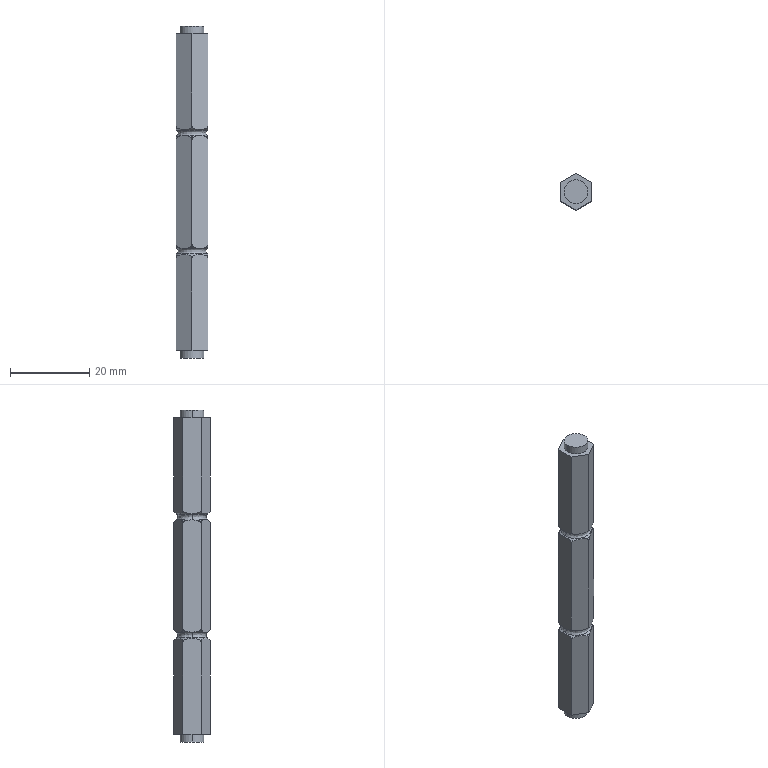Part | STEP file | 1 solid | 62 faces | box 8 x 9.238 x 84 mm | volume 4502 mm3 | spline 28 | plane 22 | cone 8 | cylinder 4 | commonest cylinder face diameters 6 x4